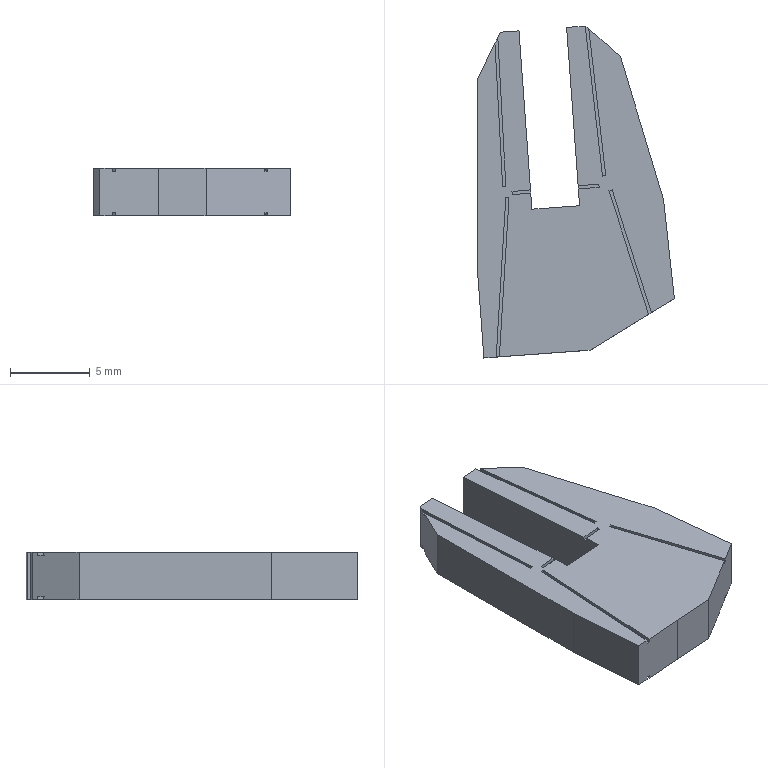Part | SolidWorks | features BaseBody 1 | 1 solid | 64 faces | box 12.359 x 20.834 x 3 mm | volume 528.554 mm3 | plane 54 | spline 10